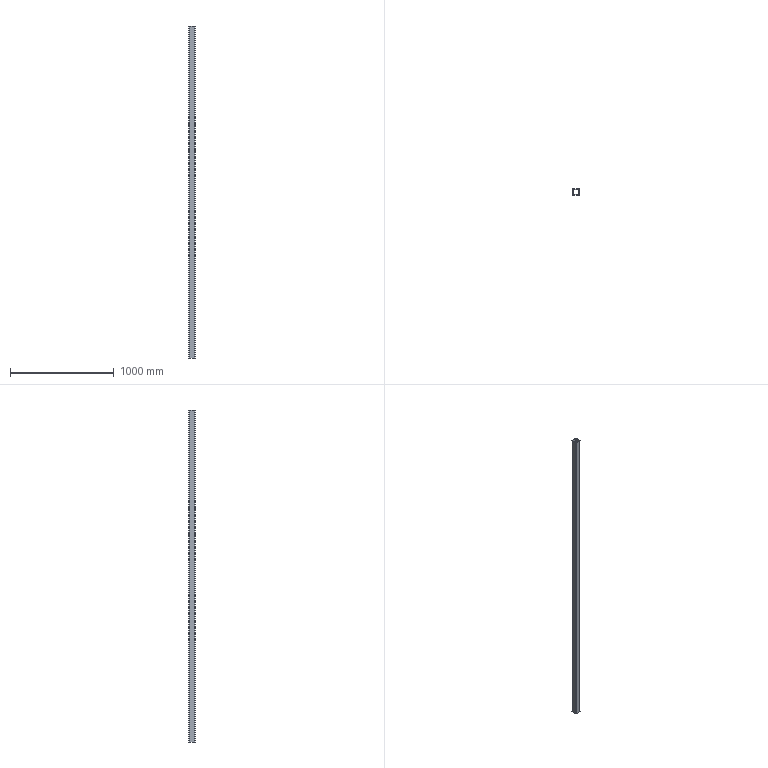Part | STEP file | 750038157 | 1 solid | 18 faces | box 60 x 60 x 3195 mm | volume 2774956 mm3 | plane 10 | cylinder 8 | commonest cylinder face diameters 4 x4 12 x4
STEP:
#1=CARTESIAN_POINT('',(-26.,24.,3195.));
#2=VERTEX_POINT('',#1);
#3=CARTESIAN_POINT('',(-26.,24.,0.));
#4=VERTEX_POINT('',#3);
#5=CARTESIAN_POINT('',(-26.,24.,3195.));
#6=DIRECTION('',(0.,0.,-1.));
#7=VECTOR('',#6,1000.);
#8=LINE('',#5,#7);
#9=EDGE_CURVE('',#2,#4,#8,.T.);
#10=ORIENTED_EDGE('',*,*,#9,.F.);
#11=CARTESIAN_POINT('',(-26.,-24.,3195.));
#12=VERTEX_POINT('',#11);
#13=CARTESIAN_POINT('',(-26.,-24.,3195.));
#14=DIRECTION('',(0.,1.,0.));
#15=VECTOR('',#14,1000.);
#16=LINE('',#13,#15);
#17=EDGE_CURVE('',#12,#2,#16,.T.);
#18=ORIENTED_EDGE('',*,*,#17,.F.);
#19=CARTESIAN_POINT('',(-26.,-24.,0.));
#20=VERTEX_POINT('',#19);
#21=CARTESIAN_POINT('',(-26.,-24.,3195.));
#22=DIRECTION('',(0.,0.,1.));
#23=VECTOR('',#22,1000.);
#24=LINE('',#21,#23);
#25=EDGE_CURVE('',#20,#12,#24,.T.);
#26=ORIENTED_EDGE('',*,*,#25,.F.);
#27=CARTESIAN_POINT('',(-26.,-24.,0.));
#28=DIRECTION('',(0.,-1.,0.));
#29=VECTOR('',#28,1000.);
#30=LINE('',#27,#29);
#31=EDGE_CURVE('',#4,#20,#30,.T.);
#32=ORIENTED_EDGE('',*,*,#31,.F.);
#33=EDGE_LOOP('',(#10,#18,#26,#32));
#34=FACE_OUTER_BOUND('',#33,.T.);
#35=CARTESIAN_POINT('',(-26.,-24.,3195.));
#36=DIRECTION('',(-1.,0.,0.));
#37=DIRECTION('',(0.,-1.,0.));
#38=AXIS2_PLACEMENT_3D('',#35,#36,#37);
#39=PLANE('',#38);
#40=ADVANCED_FACE('',(#34),#39,.F.);
#41=CARTESIAN_POINT('',(26.,24.,0.));
#42=VERTEX_POINT('',#41);
#43=CARTESIAN_POINT('',(24.,26.,0.));
#44=VERTEX_POINT('',#43);
#45=CARTESIAN_POINT('',(24.,24.,0.));
#46=DIRECTION('',(0.,0.,1.));
#47=DIRECTION('',(-1.,0.,0.));
#48=AXIS2_PLACEMENT_3D('',#45,#46,#47);
#49=CIRCLE('',#48,2.);
#50=EDGE_CURVE('',#42,#44,#49,.T.);
#51=ORIENTED_EDGE('',*,*,#50,.T.);
#52=CARTESIAN_POINT('',(-24.,26.,0.));
#53=VERTEX_POINT('',#52);
#54=CARTESIAN_POINT('',(24.,26.,0.));
#55=DIRECTION('',(-1.,0.,0.));
#56=VECTOR('',#55,1000.);
#57=LINE('',#54,#56);
#58=EDGE_CURVE('',#44,#53,#57,.T.);
#59=ORIENTED_EDGE('',*,*,#58,.T.);
#60=CARTESIAN_POINT('',(-24.,24.,0.));
#61=DIRECTION('',(0.,0.,1.));
#62=DIRECTION('',(-1.,0.,0.));
#63=AXIS2_PLACEMENT_3D('',#60,#61,#62);
#64=CIRCLE('',#63,2.);
#65=EDGE_CURVE('',#53,#4,#64,.T.);
#66=ORIENTED_EDGE('',*,*,#65,.T.);
#67=ORIENTED_EDGE('',*,*,#31,.T.);
#68=CARTESIAN_POINT('',(-24.,-26.,0.));
#69=VERTEX_POINT('',#68);
#70=CARTESIAN_POINT('',(-24.,-24.,0.));
#71=DIRECTION('',(0.,0.,1.));
#72=DIRECTION('',(-1.,0.,0.));
#73=AXIS2_PLACEMENT_3D('',#70,#71,#72);
#74=CIRCLE('',#73,2.);
#75=EDGE_CURVE('',#20,#69,#74,.T.);
#76=ORIENTED_EDGE('',*,*,#75,.T.);
#77=CARTESIAN_POINT('',(24.,-26.,0.));
#78=VERTEX_POINT('',#77);
#79=CARTESIAN_POINT('',(24.,-26.,0.));
#80=DIRECTION('',(1.,0.,0.));
#81=VECTOR('',#80,1000.);
#82=LINE('',#79,#81);
#83=EDGE_CURVE('',#69,#78,#82,.T.);
#84=ORIENTED_EDGE('',*,*,#83,.T.);
#85=CARTESIAN_POINT('',(26.,-24.,0.));
#86=VERTEX_POINT('',#85);
#87=CARTESIAN_POINT('',(24.,-24.,0.));
#88=DIRECTION('',(0.,0.,1.));
#89=DIRECTION('',(-1.,0.,0.));
#90=AXIS2_PLACEMENT_3D('',#87,#88,#89);
#91=CIRCLE('',#90,2.);
#92=EDGE_CURVE('',#78,#86,#91,.T.);
#93=ORIENTED_EDGE('',*,*,#92,.T.);
#94=CARTESIAN_POINT('',(26.,-24.,0.));
#95=DIRECTION('',(0.,1.,0.));
#96=VECTOR('',#95,1000.);
#97=LINE('',#94,#96);
#98=EDGE_CURVE('',#86,#42,#97,.T.);
#99=ORIENTED_EDGE('',*,*,#98,.T.);
#100=EDGE_LOOP('',(#51,#59,#66,#67,#76,#84,#93,#99));
#101=FACE_BOUND('',#100,.T.);
#102=CARTESIAN_POINT('',(-24.,30.,0.));
#103=VERTEX_POINT('',#102);
#104=CARTESIAN_POINT('',(24.,30.,0.));
#105=VERTEX_POINT('',#104);
#106=CARTESIAN_POINT('',(24.,30.,0.));
#107=DIRECTION('',(1.,0.,0.));
#108=VECTOR('',#107,1000.);
#109=LINE('',#106,#108);
#110=EDGE_CURVE('',#103,#105,#109,.T.);
#111=ORIENTED_EDGE('',*,*,#110,.T.);
#112=CARTESIAN_POINT('',(30.,24.,0.));
#113=VERTEX_POINT('',#112);
#114=CARTESIAN_POINT('',(24.,24.,0.));
#115=DIRECTION('',(0.,0.,-1.));
#116=DIRECTION('',(-1.,0.,0.));
#117=AXIS2_PLACEMENT_3D('',#114,#115,#116);
#118=CIRCLE('',#117,6.);
#119=EDGE_CURVE('',#105,#113,#118,.T.);
#120=ORIENTED_EDGE('',*,*,#119,.T.);
#121=CARTESIAN_POINT('',(30.,-24.,0.));
#122=VERTEX_POINT('',#121);
#123=CARTESIAN_POINT('',(30.,-24.,0.));
#124=DIRECTION('',(0.,-1.,0.));
#125=VECTOR('',#124,1000.);
#126=LINE('',#123,#125);
#127=EDGE_CURVE('',#113,#122,#126,.T.);
#128=ORIENTED_EDGE('',*,*,#127,.T.);
#129=CARTESIAN_POINT('',(24.,-30.,0.));
#130=VERTEX_POINT('',#129);
#131=CARTESIAN_POINT('',(24.,-24.,0.));
#132=DIRECTION('',(0.,0.,-1.));
#133=DIRECTION('',(-1.,0.,0.));
#134=AXIS2_PLACEMENT_3D('',#131,#132,#133);
#135=CIRCLE('',#134,6.);
#136=EDGE_CURVE('',#122,#130,#135,.T.);
#137=ORIENTED_EDGE('',*,*,#136,.T.);
#138=CARTESIAN_POINT('',(-24.,-30.,0.));
#139=VERTEX_POINT('',#138);
#140=CARTESIAN_POINT('',(24.,-30.,0.));
#141=DIRECTION('',(-1.,0.,0.));
#142=VECTOR('',#141,1000.);
#143=LINE('',#140,#142);
#144=EDGE_CURVE('',#130,#139,#143,.T.);
#145=ORIENTED_EDGE('',*,*,#144,.T.);
#146=CARTESIAN_POINT('',(-30.,-24.,0.));
#147=VERTEX_POINT('',#146);
#148=CARTESIAN_POINT('',(-24.,-24.,0.));
#149=DIRECTION('',(0.,0.,-1.));
#150=DIRECTION('',(-1.,0.,0.));
#151=AXIS2_PLACEMENT_3D('',#148,#149,#150);
#152=CIRCLE('',#151,6.);
#153=EDGE_CURVE('',#139,#147,#152,.T.);
#154=ORIENTED_EDGE('',*,*,#153,.T.);
#155=CARTESIAN_POINT('',(-30.,24.,0.));
#156=VERTEX_POINT('',#155);
#157=CARTESIAN_POINT('',(-30.,-24.,0.));
#158=DIRECTION('',(0.,1.,0.));
#159=VECTOR('',#158,1000.);
#160=LINE('',#157,#159);
#161=EDGE_CURVE('',#147,#156,#160,.T.);
#162=ORIENTED_EDGE('',*,*,#161,.T.);
#163=CARTESIAN_POINT('',(-24.,24.,0.));
#164=DIRECTION('',(0.,0.,-1.));
#165=DIRECTION('',(-1.,0.,0.));
#166=AXIS2_PLACEMENT_3D('',#163,#164,#165);
#167=CIRCLE('',#166,6.);
#168=EDGE_CURVE('',#156,#103,#167,.T.);
#169=ORIENTED_EDGE('',*,*,#168,.T.);
#170=EDGE_LOOP('',(#111,#120,#128,#137,#145,#154,#162,#169));
#171=FACE_OUTER_BOUND('',#170,.T.);
#172=CARTESIAN_POINT('',(24.,-24.,0.));
#173=DIRECTION('',(0.,0.,-1.));
#174=DIRECTION('',(-1.,0.,0.));
#175=AXIS2_PLACEMENT_3D('',#172,#173,#174);
#176=PLANE('',#175);
#177=ADVANCED_FACE('',(#101,#171),#176,.T.);
#178=CARTESIAN_POINT('',(-24.,26.,3195.));
#179=VERTEX_POINT('',#178);
#180=CARTESIAN_POINT('',(-24.,26.,3195.));
#181=DIRECTION('',(0.,0.,-1.));
#182=VECTOR('',#181,1000.);
#183=LINE('',#180,#182);
#184=EDGE_CURVE('',#179,#53,#183,.T.);
#185=ORIENTED_EDGE('',*,*,#184,.F.);
#186=CARTESIAN_POINT('',(-24.,24.,3195.));
#187=DIRECTION('',(0.,0.,-1.));
#188=DIRECTION('',(-1.,0.,0.));
#189=AXIS2_PLACEMENT_3D('',#186,#187,#188);
#190=CIRCLE('',#189,2.);
#191=EDGE_CURVE('',#2,#179,#190,.T.);
#192=ORIENTED_EDGE('',*,*,#191,.F.);
#193=ORIENTED_EDGE('',*,*,#9,.T.);
#194=ORIENTED_EDGE('',*,*,#65,.F.);
#195=EDGE_LOOP('',(#185,#192,#193,#194));
#196=FACE_OUTER_BOUND('',#195,.T.);
#197=CARTESIAN_POINT('',(-24.,24.,3195.));
#198=DIRECTION('',(0.,0.,-1.));
#199=DIRECTION('',(-1.,0.,0.));
#200=AXIS2_PLACEMENT_3D('',#197,#198,#199);
#201=CYLINDRICAL_SURFACE('',#200,2.);
#202=ADVANCED_FACE('',(#196),#201,.F.);
#203=CARTESIAN_POINT('',(24.,26.,3195.));
#204=VERTEX_POINT('',#203);
#205=CARTESIAN_POINT('',(24.,26.,3195.));
#206=DIRECTION('',(-1.,0.,0.));
#207=VECTOR('',#206,1000.);
#208=LINE('',#205,#207);
#209=EDGE_CURVE('',#204,#179,#208,.T.);
#210=ORIENTED_EDGE('',*,*,#209,.F.);
#211=CARTESIAN_POINT('',(26.,24.,3195.));
#212=VERTEX_POINT('',#211);
#213=CARTESIAN_POINT('',(24.,24.,3195.));
#214=DIRECTION('',(0.,0.,1.));
#215=DIRECTION('',(-1.,0.,0.));
#216=AXIS2_PLACEMENT_3D('',#213,#214,#215);
#217=CIRCLE('',#216,2.);
#218=EDGE_CURVE('',#212,#204,#217,.T.);
#219=ORIENTED_EDGE('',*,*,#218,.F.);
#220=CARTESIAN_POINT('',(26.,-24.,3195.));
#221=VERTEX_POINT('',#220);
#222=CARTESIAN_POINT('',(26.,-24.,3195.));
#223=DIRECTION('',(0.,1.,0.));
#224=VECTOR('',#223,1000.);
#225=LINE('',#222,#224);
#226=EDGE_CURVE('',#221,#212,#225,.T.);
#227=ORIENTED_EDGE('',*,*,#226,.F.);
#228=CARTESIAN_POINT('',(24.,-26.,3195.));
#229=VERTEX_POINT('',#228);
#230=CARTESIAN_POINT('',(24.,-24.,3195.));
#231=DIRECTION('',(0.,0.,1.));
#232=DIRECTION('',(-1.,0.,0.));
#233=AXIS2_PLACEMENT_3D('',#230,#231,#232);
#234=CIRCLE('',#233,2.);
#235=EDGE_CURVE('',#229,#221,#234,.T.);
#236=ORIENTED_EDGE('',*,*,#235,.F.);
#237=CARTESIAN_POINT('',(-24.,-26.,3195.));
#238=VERTEX_POINT('',#237);
#239=CARTESIAN_POINT('',(24.,-26.,3195.));
#240=DIRECTION('',(1.,0.,0.));
#241=VECTOR('',#240,1000.);
#242=LINE('',#239,#241);
#243=EDGE_CURVE('',#238,#229,#242,.T.);
#244=ORIENTED_EDGE('',*,*,#243,.F.);
#245=CARTESIAN_POINT('',(-24.,-24.,3195.));
#246=DIRECTION('',(0.,0.,1.));
#247=DIRECTION('',(-1.,0.,0.));
#248=AXIS2_PLACEMENT_3D('',#245,#246,#247);
#249=CIRCLE('',#248,2.);
#250=EDGE_CURVE('',#12,#238,#249,.T.);
#251=ORIENTED_EDGE('',*,*,#250,.F.);
#252=ORIENTED_EDGE('',*,*,#17,.T.);
#253=ORIENTED_EDGE('',*,*,#191,.T.);
#254=EDGE_LOOP('',(#210,#219,#227,#236,#244,#251,#252,#253));
#255=FACE_BOUND('',#254,.T.);
#256=CARTESIAN_POINT('',(24.,30.,3195.));
#257=VERTEX_POINT('',#256);
#258=CARTESIAN_POINT('',(30.,24.,3195.));
#259=VERTEX_POINT('',#258);
#260=CARTESIAN_POINT('',(24.,24.,3195.));
#261=DIRECTION('',(0.,0.,-1.));
#262=DIRECTION('',(-1.,0.,0.));
#263=AXIS2_PLACEMENT_3D('',#260,#261,#262);
#264=CIRCLE('',#263,6.);
#265=EDGE_CURVE('',#257,#259,#264,.T.);
#266=ORIENTED_EDGE('',*,*,#265,.F.);
#267=CARTESIAN_POINT('',(-24.,30.,3195.));
#268=VERTEX_POINT('',#267);
#269=CARTESIAN_POINT('',(24.,30.,3195.));
#270=DIRECTION('',(1.,0.,0.));
#271=VECTOR('',#270,1000.);
#272=LINE('',#269,#271);
#273=EDGE_CURVE('',#268,#257,#272,.T.);
#274=ORIENTED_EDGE('',*,*,#273,.F.);
#275=CARTESIAN_POINT('',(-30.,24.,3195.));
#276=VERTEX_POINT('',#275);
#277=CARTESIAN_POINT('',(-24.,24.,3195.));
#278=DIRECTION('',(0.,0.,-1.));
#279=DIRECTION('',(-1.,0.,0.));
#280=AXIS2_PLACEMENT_3D('',#277,#278,#279);
#281=CIRCLE('',#280,6.);
#282=EDGE_CURVE('',#276,#268,#281,.T.);
#283=ORIENTED_EDGE('',*,*,#282,.F.);
#284=CARTESIAN_POINT('',(-30.,-24.,3195.));
#285=VERTEX_POINT('',#284);
#286=CARTESIAN_POINT('',(-30.,-24.,3195.));
#287=DIRECTION('',(0.,1.,0.));
#288=VECTOR('',#287,1000.);
#289=LINE('',#286,#288);
#290=EDGE_CURVE('',#285,#276,#289,.T.);
#291=ORIENTED_EDGE('',*,*,#290,.F.);
#292=CARTESIAN_POINT('',(-24.,-30.,3195.));
#293=VERTEX_POINT('',#292);
#294=CARTESIAN_POINT('',(-24.,-24.,3195.));
#295=DIRECTION('',(0.,0.,-1.));
#296=DIRECTION('',(-1.,0.,0.));
#297=AXIS2_PLACEMENT_3D('',#294,#295,#296);
#298=CIRCLE('',#297,6.);
#299=EDGE_CURVE('',#293,#285,#298,.T.);
#300=ORIENTED_EDGE('',*,*,#299,.F.);
#301=CARTESIAN_POINT('',(24.,-30.,3195.));
#302=VERTEX_POINT('',#301);
#303=CARTESIAN_POINT('',(24.,-30.,3195.));
#304=DIRECTION('',(-1.,0.,0.));
#305=VECTOR('',#304,1000.);
#306=LINE('',#303,#305);
#307=EDGE_CURVE('',#302,#293,#306,.T.);
#308=ORIENTED_EDGE('',*,*,#307,.F.);
#309=CARTESIAN_POINT('',(30.,-24.,3195.));
#310=VERTEX_POINT('',#309);
#311=CARTESIAN_POINT('',(24.,-24.,3195.));
#312=DIRECTION('',(0.,0.,-1.));
#313=DIRECTION('',(-1.,0.,0.));
#314=AXIS2_PLACEMENT_3D('',#311,#312,#313);
#315=CIRCLE('',#314,6.);
#316=EDGE_CURVE('',#310,#302,#315,.T.);
#317=ORIENTED_EDGE('',*,*,#316,.F.);
#318=CARTESIAN_POINT('',(30.,-24.,3195.));
#319=DIRECTION('',(0.,-1.,0.));
#320=VECTOR('',#319,1000.);
#321=LINE('',#318,#320);
#322=EDGE_CURVE('',#259,#310,#321,.T.);
#323=ORIENTED_EDGE('',*,*,#322,.F.);
#324=EDGE_LOOP('',(#266,#274,#283,#291,#300,#308,#317,#323));
#325=FACE_OUTER_BOUND('',#324,.T.);
#326=CARTESIAN_POINT('',(24.,-24.,3195.));
#327=DIRECTION('',(0.,0.,-1.));
#328=DIRECTION('',(-1.,0.,0.));
#329=AXIS2_PLACEMENT_3D('',#326,#327,#328);
#330=PLANE('',#329);
#331=ADVANCED_FACE('',(#255,#325),#330,.F.);
#332=ORIENTED_EDGE('',*,*,#25,.T.);
#333=ORIENTED_EDGE('',*,*,#250,.T.);
#334=CARTESIAN_POINT('',(-24.,-26.,3195.));
#335=DIRECTION('',(0.,0.,1.));
#336=VECTOR('',#335,1000.);
#337=LINE('',#334,#336);
#338=EDGE_CURVE('',#69,#238,#337,.T.);
#339=ORIENTED_EDGE('',*,*,#338,.F.);
#340=ORIENTED_EDGE('',*,*,#75,.F.);
#341=EDGE_LOOP('',(#332,#333,#339,#340));
#342=FACE_OUTER_BOUND('',#341,.T.);
#343=CARTESIAN_POINT('',(-24.,-24.,3195.));
#344=DIRECTION('',(0.,0.,-1.));
#345=DIRECTION('',(-1.,0.,0.));
#346=AXIS2_PLACEMENT_3D('',#343,#344,#345);
#347=CYLINDRICAL_SURFACE('',#346,2.);
#348=ADVANCED_FACE('',(#342),#347,.F.);
#349=CARTESIAN_POINT('',(24.,26.,3195.));
#350=DIRECTION('',(0.,0.,-1.));
#351=VECTOR('',#350,1000.);
#352=LINE('',#349,#351);
#353=EDGE_CURVE('',#204,#44,#352,.T.);
#354=ORIENTED_EDGE('',*,*,#353,.F.);
#355=ORIENTED_EDGE('',*,*,#209,.T.);
#356=ORIENTED_EDGE('',*,*,#184,.T.);
#357=ORIENTED_EDGE('',*,*,#58,.F.);
#358=EDGE_LOOP('',(#354,#355,#356,#357));
#359=FACE_OUTER_BOUND('',#358,.T.);
#360=CARTESIAN_POINT('',(-24.,26.,3195.));
#361=DIRECTION('',(0.,1.,0.));
#362=DIRECTION('',(0.,0.,1.));
#363=AXIS2_PLACEMENT_3D('',#360,#361,#362);
#364=PLANE('',#363);
#365=ADVANCED_FACE('',(#359),#364,.F.);
#366=CARTESIAN_POINT('',(26.,24.,3195.));
#367=DIRECTION('',(0.,0.,-1.));
#368=VECTOR('',#367,1000.);
#369=LINE('',#366,#368);
#370=EDGE_CURVE('',#212,#42,#369,.T.);
#371=ORIENTED_EDGE('',*,*,#370,.F.);
#372=ORIENTED_EDGE('',*,*,#218,.T.);
#373=ORIENTED_EDGE('',*,*,#353,.T.);
#374=ORIENTED_EDGE('',*,*,#50,.F.);
#375=EDGE_LOOP('',(#371,#372,#373,#374));
#376=FACE_OUTER_BOUND('',#375,.T.);
#377=CARTESIAN_POINT('',(24.,24.,3195.));
#378=DIRECTION('',(0.,0.,-1.));
#379=DIRECTION('',(-1.,0.,0.));
#380=AXIS2_PLACEMENT_3D('',#377,#378,#379);
#381=CYLINDRICAL_SURFACE('',#380,2.);
#382=ADVANCED_FACE('',(#376),#381,.F.);
#383=CARTESIAN_POINT('',(26.,-24.,3195.));
#384=DIRECTION('',(0.,0.,-1.));
#385=VECTOR('',#384,1000.);
#386=LINE('',#383,#385);
#387=EDGE_CURVE('',#221,#86,#386,.T.);
#388=ORIENTED_EDGE('',*,*,#387,.F.);
#389=ORIENTED_EDGE('',*,*,#226,.T.);
#390=ORIENTED_EDGE('',*,*,#370,.T.);
#391=ORIENTED_EDGE('',*,*,#98,.F.);
#392=EDGE_LOOP('',(#388,#389,#390,#391));
#393=FACE_OUTER_BOUND('',#392,.T.);
#394=CARTESIAN_POINT('',(26.,24.,3195.));
#395=DIRECTION('',(1.,0.,0.));
#396=DIRECTION('',(0.,0.,-1.));
#397=AXIS2_PLACEMENT_3D('',#394,#395,#396);
#398=PLANE('',#397);
#399=ADVANCED_FACE('',(#393),#398,.F.);
#400=CARTESIAN_POINT('',(24.,-26.,3195.));
#401=DIRECTION('',(0.,0.,-1.));
#402=VECTOR('',#401,1000.);
#403=LINE('',#400,#402);
#404=EDGE_CURVE('',#229,#78,#403,.T.);
#405=ORIENTED_EDGE('',*,*,#404,.F.);
#406=ORIENTED_EDGE('',*,*,#235,.T.);
#407=ORIENTED_EDGE('',*,*,#387,.T.);
#408=ORIENTED_EDGE('',*,*,#92,.F.);
#409=EDGE_LOOP('',(#405,#406,#407,#408));
#410=FACE_OUTER_BOUND('',#409,.T.);
#411=CARTESIAN_POINT('',(24.,-24.,3195.));
#412=DIRECTION('',(0.,0.,-1.));
#413=DIRECTION('',(-1.,0.,0.));
#414=AXIS2_PLACEMENT_3D('',#411,#412,#413);
#415=CYLINDRICAL_SURFACE('',#414,2.);
#416=ADVANCED_FACE('',(#410),#415,.F.);
#417=ORIENTED_EDGE('',*,*,#338,.T.);
#418=ORIENTED_EDGE('',*,*,#243,.T.);
#419=ORIENTED_EDGE('',*,*,#404,.T.);
#420=ORIENTED_EDGE('',*,*,#83,.F.);
#421=EDGE_LOOP('',(#417,#418,#419,#420));
#422=FACE_OUTER_BOUND('',#421,.T.);
#423=CARTESIAN_POINT('',(24.,-26.,3195.));
#424=DIRECTION('',(0.,-1.,0.));
#425=DIRECTION('',(0.,0.,-1.));
#426=AXIS2_PLACEMENT_3D('',#423,#424,#425);
#427=PLANE('',#426);
#428=ADVANCED_FACE('',(#422),#427,.F.);
#429=ORIENTED_EDGE('',*,*,#265,.T.);
#430=CARTESIAN_POINT('',(30.,24.,3195.));
#431=DIRECTION('',(0.,0.,-1.));
#432=VECTOR('',#431,1000.);
#433=LINE('',#430,#432);
#434=EDGE_CURVE('',#259,#113,#433,.T.);
#435=ORIENTED_EDGE('',*,*,#434,.T.);
#436=ORIENTED_EDGE('',*,*,#119,.F.);
#437=CARTESIAN_POINT('',(24.,30.,3195.));
#438=DIRECTION('',(0.,0.,1.));
#439=VECTOR('',#438,1000.);
#440=LINE('',#437,#439);
#441=EDGE_CURVE('',#105,#257,#440,.T.);
#442=ORIENTED_EDGE('',*,*,#441,.T.);
#443=EDGE_LOOP('',(#429,#435,#436,#442));
#444=FACE_OUTER_BOUND('',#443,.T.);
#445=CARTESIAN_POINT('',(24.,24.,3195.));
#446=DIRECTION('',(0.,0.,-1.));
#447=DIRECTION('',(-1.,0.,0.));
#448=AXIS2_PLACEMENT_3D('',#445,#446,#447);
#449=CYLINDRICAL_SURFACE('',#448,6.);
#450=ADVANCED_FACE('',(#444),#449,.T.);
#451=ORIENTED_EDGE('',*,*,#273,.T.);
#452=ORIENTED_EDGE('',*,*,#441,.F.);
#453=ORIENTED_EDGE('',*,*,#110,.F.);
#454=CARTESIAN_POINT('',(-24.,30.,3195.));
#455=DIRECTION('',(0.,0.,1.));
#456=VECTOR('',#455,1000.);
#457=LINE('',#454,#456);
#458=EDGE_CURVE('',#103,#268,#457,.T.);
#459=ORIENTED_EDGE('',*,*,#458,.T.);
#460=EDGE_LOOP('',(#451,#452,#453,#459));
#461=FACE_OUTER_BOUND('',#460,.T.);
#462=CARTESIAN_POINT('',(-24.,30.,3195.));
#463=DIRECTION('',(0.,1.,0.));
#464=DIRECTION('',(-1.,0.,0.));
#465=AXIS2_PLACEMENT_3D('',#462,#463,#464);
#466=PLANE('',#465);
#467=ADVANCED_FACE('',(#461),#466,.T.);
#468=ORIENTED_EDGE('',*,*,#282,.T.);
#469=ORIENTED_EDGE('',*,*,#458,.F.);
#470=ORIENTED_EDGE('',*,*,#168,.F.);
#471=CARTESIAN_POINT('',(-30.,24.,3195.));
#472=DIRECTION('',(0.,0.,1.));
#473=VECTOR('',#472,1000.);
#474=LINE('',#471,#473);
#475=EDGE_CURVE('',#156,#276,#474,.T.);
#476=ORIENTED_EDGE('',*,*,#475,.T.);
#477=EDGE_LOOP('',(#468,#469,#470,#476));
#478=FACE_OUTER_BOUND('',#477,.T.);
#479=CARTESIAN_POINT('',(-24.,24.,3195.));
#480=DIRECTION('',(0.,0.,-1.));
#481=DIRECTION('',(-1.,0.,0.));
#482=AXIS2_PLACEMENT_3D('',#479,#480,#481);
#483=CYLINDRICAL_SURFACE('',#482,6.);
#484=ADVANCED_FACE('',(#478),#483,.T.);
#485=ORIENTED_EDGE('',*,*,#290,.T.);
#486=ORIENTED_EDGE('',*,*,#475,.F.);
#487=ORIENTED_EDGE('',*,*,#161,.F.);
#488=CARTESIAN_POINT('',(-30.,-24.,3195.));
#489=DIRECTION('',(0.,0.,1.));
#490=VECTOR('',#489,1000.);
#491=LINE('',#488,#490);
#492=EDGE_CURVE('',#147,#285,#491,.T.);
#493=ORIENTED_EDGE('',*,*,#492,.T.);
#494=EDGE_LOOP('',(#485,#486,#487,#493));
#495=FACE_OUTER_BOUND('',#494,.T.);
#496=CARTESIAN_POINT('',(-30.,-24.,3195.));
#497=DIRECTION('',(-1.,0.,0.));
#498=DIRECTION('',(0.,-1.,0.));
#499=AXIS2_PLACEMENT_3D('',#496,#497,#498);
#500=PLANE('',#499);
#501=ADVANCED_FACE('',(#495),#500,.T.);
#502=ORIENTED_EDGE('',*,*,#299,.T.);
#503=ORIENTED_EDGE('',*,*,#492,.F.);
#504=ORIENTED_EDGE('',*,*,#153,.F.);
#505=CARTESIAN_POINT('',(-24.,-30.,3195.));
#506=DIRECTION('',(0.,0.,1.));
#507=VECTOR('',#506,1000.);
#508=LINE('',#505,#507);
#509=EDGE_CURVE('',#139,#293,#508,.T.);
#510=ORIENTED_EDGE('',*,*,#509,.T.);
#511=EDGE_LOOP('',(#502,#503,#504,#510));
#512=FACE_OUTER_BOUND('',#511,.T.);
#513=CARTESIAN_POINT('',(-24.,-24.,3195.));
#514=DIRECTION('',(0.,0.,-1.));
#515=DIRECTION('',(-1.,0.,0.));
#516=AXIS2_PLACEMENT_3D('',#513,#514,#515);
#517=CYLINDRICAL_SURFACE('',#516,6.);
#518=ADVANCED_FACE('',(#512),#517,.T.);
#519=ORIENTED_EDGE('',*,*,#307,.T.);
#520=ORIENTED_EDGE('',*,*,#509,.F.);
#521=ORIENTED_EDGE('',*,*,#144,.F.);
#522=CARTESIAN_POINT('',(24.,-30.,3195.));
#523=DIRECTION('',(0.,0.,1.));
#524=VECTOR('',#523,1000.);
#525=LINE('',#522,#524);
#526=EDGE_CURVE('',#130,#302,#525,.T.);
#527=ORIENTED_EDGE('',*,*,#526,.T.);
#528=EDGE_LOOP('',(#519,#520,#521,#527));
#529=FACE_OUTER_BOUND('',#528,.T.);
#530=CARTESIAN_POINT('',(24.,-30.,3195.));
#531=DIRECTION('',(0.,-1.,0.));
#532=DIRECTION('',(1.,0.,0.));
#533=AXIS2_PLACEMENT_3D('',#530,#531,#532);
#534=PLANE('',#533);
#535=ADVANCED_FACE('',(#529),#534,.T.);
#536=ORIENTED_EDGE('',*,*,#316,.T.);
#537=ORIENTED_EDGE('',*,*,#526,.F.);
#538=ORIENTED_EDGE('',*,*,#136,.F.);
#539=CARTESIAN_POINT('',(30.,-24.,3195.));
#540=DIRECTION('',(0.,0.,1.));
#541=VECTOR('',#540,1000.);
#542=LINE('',#539,#541);
#543=EDGE_CURVE('',#122,#310,#542,.T.);
#544=ORIENTED_EDGE('',*,*,#543,.T.);
#545=EDGE_LOOP('',(#536,#537,#538,#544));
#546=FACE_OUTER_BOUND('',#545,.T.);
#547=CARTESIAN_POINT('',(24.,-24.,3195.));
#548=DIRECTION('',(0.,0.,-1.));
#549=DIRECTION('',(-1.,0.,0.));
#550=AXIS2_PLACEMENT_3D('',#547,#548,#549);
#551=CYLINDRICAL_SURFACE('',#550,6.);
#552=ADVANCED_FACE('',(#546),#551,.T.);
#553=ORIENTED_EDGE('',*,*,#322,.T.);
#554=ORIENTED_EDGE('',*,*,#543,.F.);
#555=ORIENTED_EDGE('',*,*,#127,.F.);
#556=ORIENTED_EDGE('',*,*,#434,.F.);
#557=EDGE_LOOP('',(#553,#554,#555,#556));
#558=FACE_OUTER_BOUND('',#557,.T.);
#559=CARTESIAN_POINT('',(30.,24.,3195.));
#560=DIRECTION('',(1.,0.,0.));
#561=DIRECTION('',(0.,0.,-1.));
#562=AXIS2_PLACEMENT_3D('',#559,#560,#561);
#563=PLANE('',#562);
#564=ADVANCED_FACE('',(#558),#563,.T.);
#565=CLOSED_SHELL('',(#40,#177,#202,#331,#348,#365,#382,#399,#416,#428,#450,#467,#484,#501,#518,#535,#552,#564));
#566=MANIFOLD_SOLID_BREP('',#565);
#567=CARTESIAN_POINT('',(0.,0.,0.));
#568=DIRECTION('',(0.,0.,1.));
#569=DIRECTION('',(1.,0.,0.));
#570=AXIS2_PLACEMENT_3D('',#567,#568,#569);
#571=(LENGTH_UNIT()NAMED_UNIT(*)SI_UNIT(.MILLI.,.METRE.));
#572=UNCERTAINTY_MEASURE_WITH_UNIT(LENGTH_MEASURE(0.00001),#571,'','');
#573=(NAMED_UNIT(*)PLANE_ANGLE_UNIT()SI_UNIT($,.RADIAN.));
#574=(NAMED_UNIT(*)SI_UNIT($,.STERADIAN.)SOLID_ANGLE_UNIT());
#575=(GEOMETRIC_REPRESENTATION_CONTEXT(3)GLOBAL_UNCERTAINTY_ASSIGNED_CONTEXT((#572))GLOBAL_UNIT_ASSIGNED_CONTEXT((#571,#573,#574))REPRESENTATION_CONTEXT('',''));
#576=ADVANCED_BREP_SHAPE_REPRESENTATION('',(#566,#570),#575);